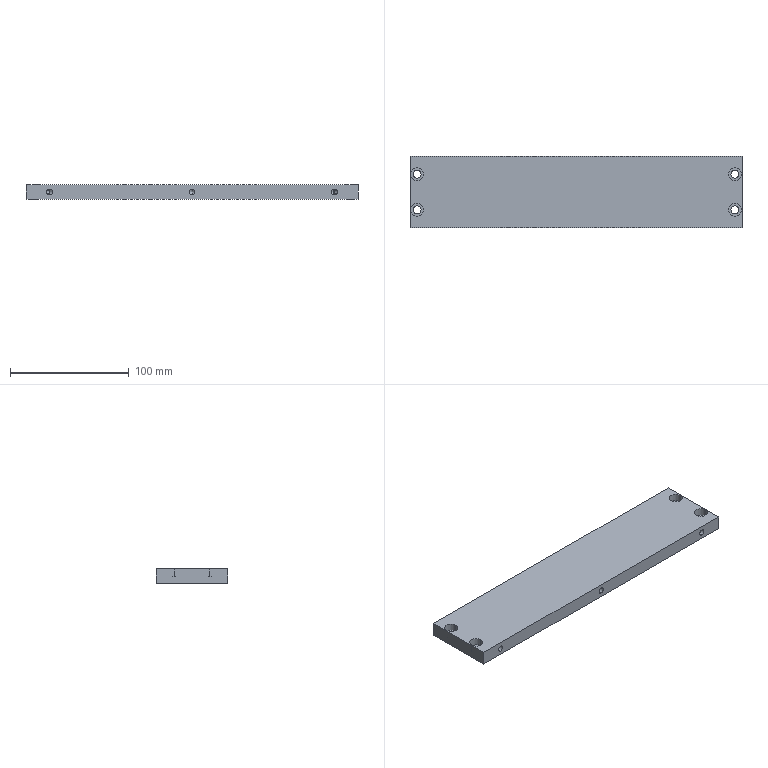Part | SolidWorks | features HoleWzd 3, Extrusion 1 | 1 solid | 50 faces | box 280 x 60 x 12 mm | volume 196575 mm3 | cylinder 28 | cone 12 | plane 10 | commonest cylinder face diameters 5 x12 6.6 x8 11 x8
STEP:
#1=CARTESIAN_POINT('',(268.5,-45.,5.6));
#2=VERTEX_POINT('',#1);
#3=CARTESIAN_POINT('',(279.5,-45.,5.6));
#4=VERTEX_POINT('',#3);
#5=CARTESIAN_POINT('',(274.,-45.,5.6));
#6=DIRECTION('',(0.,0.,1.));
#7=DIRECTION('',(1.,0.,0.));
#8=AXIS2_PLACEMENT_3D('',#5,#6,#7);
#9=CIRCLE('',#8,5.5);
#10=EDGE_CURVE('',#2,#4,#9,.T.);
#11=ORIENTED_EDGE('',*,*,#10,.F.);
#12=CARTESIAN_POINT('',(268.5,-45.,12.));
#13=VERTEX_POINT('',#12);
#14=CARTESIAN_POINT('',(268.5,-45.,12.));
#15=DIRECTION('',(0.,0.,1.));
#16=VECTOR('',#15,1000.);
#17=LINE('',#14,#16);
#18=EDGE_CURVE('',#2,#13,#17,.T.);
#19=ORIENTED_EDGE('',*,*,#18,.T.);
#20=CARTESIAN_POINT('',(279.5,-45.,12.));
#21=VERTEX_POINT('',#20);
#22=CARTESIAN_POINT('',(274.,-45.,12.));
#23=DIRECTION('',(0.,0.,1.));
#24=DIRECTION('',(1.,0.,0.));
#25=AXIS2_PLACEMENT_3D('',#22,#23,#24);
#26=CIRCLE('',#25,5.5);
#27=EDGE_CURVE('',#13,#21,#26,.T.);
#28=ORIENTED_EDGE('',*,*,#27,.T.);
#29=CARTESIAN_POINT('',(279.5,-45.,12.));
#30=DIRECTION('',(0.,0.,1.));
#31=VECTOR('',#30,1000.);
#32=LINE('',#29,#31);
#33=EDGE_CURVE('',#4,#21,#32,.T.);
#34=ORIENTED_EDGE('',*,*,#33,.F.);
#35=EDGE_LOOP('',(#11,#19,#28,#34));
#36=FACE_OUTER_BOUND('',#35,.T.);
#37=CARTESIAN_POINT('',(274.,-45.,12.));
#38=DIRECTION('',(0.,0.,1.));
#39=DIRECTION('',(1.,0.,0.));
#40=AXIS2_PLACEMENT_3D('',#37,#38,#39);
#41=CYLINDRICAL_SURFACE('',#40,5.5);
#42=ADVANCED_FACE('',(#36),#41,.F.);
#43=CARTESIAN_POINT('',(270.7,-45.,0.));
#44=VERTEX_POINT('',#43);
#45=CARTESIAN_POINT('',(277.3,-45.,0.));
#46=VERTEX_POINT('',#45);
#47=CARTESIAN_POINT('',(274.,-45.,0.));
#48=DIRECTION('',(0.,0.,1.));
#49=DIRECTION('',(1.,0.,0.));
#50=AXIS2_PLACEMENT_3D('',#47,#48,#49);
#51=CIRCLE('',#50,3.3);
#52=EDGE_CURVE('',#44,#46,#51,.T.);
#53=ORIENTED_EDGE('',*,*,#52,.F.);
#54=CARTESIAN_POINT('',(270.7,-45.,5.6));
#55=VERTEX_POINT('',#54);
#56=CARTESIAN_POINT('',(270.7,-45.,12.));
#57=DIRECTION('',(0.,0.,1.));
#58=VECTOR('',#57,1000.);
#59=LINE('',#56,#58);
#60=EDGE_CURVE('',#44,#55,#59,.T.);
#61=ORIENTED_EDGE('',*,*,#60,.T.);
#62=CARTESIAN_POINT('',(277.3,-45.,5.6));
#63=VERTEX_POINT('',#62);
#64=CARTESIAN_POINT('',(274.,-45.,5.6));
#65=DIRECTION('',(0.,0.,1.));
#66=DIRECTION('',(1.,0.,0.));
#67=AXIS2_PLACEMENT_3D('',#64,#65,#66);
#68=CIRCLE('',#67,3.3);
#69=EDGE_CURVE('',#55,#63,#68,.T.);
#70=ORIENTED_EDGE('',*,*,#69,.T.);
#71=CARTESIAN_POINT('',(277.3,-45.,12.));
#72=DIRECTION('',(0.,0.,1.));
#73=VECTOR('',#72,1000.);
#74=LINE('',#71,#73);
#75=EDGE_CURVE('',#46,#63,#74,.T.);
#76=ORIENTED_EDGE('',*,*,#75,.F.);
#77=EDGE_LOOP('',(#53,#61,#70,#76));
#78=FACE_OUTER_BOUND('',#77,.T.);
#79=CARTESIAN_POINT('',(274.,-45.,12.));
#80=DIRECTION('',(0.,0.,1.));
#81=DIRECTION('',(1.,0.,0.));
#82=AXIS2_PLACEMENT_3D('',#79,#80,#81);
#83=CYLINDRICAL_SURFACE('',#82,3.3);
#84=ADVANCED_FACE('',(#78),#83,.F.);
#85=CARTESIAN_POINT('',(268.5,-15.,5.6));
#86=VERTEX_POINT('',#85);
#87=CARTESIAN_POINT('',(279.5,-15.,5.6));
#88=VERTEX_POINT('',#87);
#89=CARTESIAN_POINT('',(274.,-15.,5.6));
#90=DIRECTION('',(0.,0.,1.));
#91=DIRECTION('',(1.,0.,0.));
#92=AXIS2_PLACEMENT_3D('',#89,#90,#91);
#93=CIRCLE('',#92,5.5);
#94=EDGE_CURVE('',#86,#88,#93,.T.);
#95=ORIENTED_EDGE('',*,*,#94,.F.);
#96=CARTESIAN_POINT('',(268.5,-15.,12.));
#97=VERTEX_POINT('',#96);
#98=CARTESIAN_POINT('',(268.5,-15.,12.));
#99=DIRECTION('',(0.,0.,1.));
#100=VECTOR('',#99,1000.);
#101=LINE('',#98,#100);
#102=EDGE_CURVE('',#86,#97,#101,.T.);
#103=ORIENTED_EDGE('',*,*,#102,.T.);
#104=CARTESIAN_POINT('',(279.5,-15.,12.));
#105=VERTEX_POINT('',#104);
#106=CARTESIAN_POINT('',(274.,-15.,12.));
#107=DIRECTION('',(0.,0.,1.));
#108=DIRECTION('',(1.,0.,0.));
#109=AXIS2_PLACEMENT_3D('',#106,#107,#108);
#110=CIRCLE('',#109,5.5);
#111=EDGE_CURVE('',#97,#105,#110,.T.);
#112=ORIENTED_EDGE('',*,*,#111,.T.);
#113=CARTESIAN_POINT('',(279.5,-15.,12.));
#114=DIRECTION('',(0.,0.,1.));
#115=VECTOR('',#114,1000.);
#116=LINE('',#113,#115);
#117=EDGE_CURVE('',#88,#105,#116,.T.);
#118=ORIENTED_EDGE('',*,*,#117,.F.);
#119=EDGE_LOOP('',(#95,#103,#112,#118));
#120=FACE_OUTER_BOUND('',#119,.T.);
#121=CARTESIAN_POINT('',(274.,-15.,12.));
#122=DIRECTION('',(0.,0.,1.));
#123=DIRECTION('',(1.,0.,0.));
#124=AXIS2_PLACEMENT_3D('',#121,#122,#123);
#125=CYLINDRICAL_SURFACE('',#124,5.5);
#126=ADVANCED_FACE('',(#120),#125,.F.);
#127=CARTESIAN_POINT('',(270.7,-15.,0.));
#128=VERTEX_POINT('',#127);
#129=CARTESIAN_POINT('',(277.3,-15.,0.));
#130=VERTEX_POINT('',#129);
#131=CARTESIAN_POINT('',(274.,-15.,0.));
#132=DIRECTION('',(0.,0.,1.));
#133=DIRECTION('',(1.,0.,0.));
#134=AXIS2_PLACEMENT_3D('',#131,#132,#133);
#135=CIRCLE('',#134,3.3);
#136=EDGE_CURVE('',#128,#130,#135,.T.);
#137=ORIENTED_EDGE('',*,*,#136,.F.);
#138=CARTESIAN_POINT('',(270.7,-15.,5.6));
#139=VERTEX_POINT('',#138);
#140=CARTESIAN_POINT('',(270.7,-15.,12.));
#141=DIRECTION('',(0.,0.,1.));
#142=VECTOR('',#141,1000.);
#143=LINE('',#140,#142);
#144=EDGE_CURVE('',#128,#139,#143,.T.);
#145=ORIENTED_EDGE('',*,*,#144,.T.);
#146=CARTESIAN_POINT('',(277.3,-15.,5.6));
#147=VERTEX_POINT('',#146);
#148=CARTESIAN_POINT('',(274.,-15.,5.6));
#149=DIRECTION('',(0.,0.,1.));
#150=DIRECTION('',(1.,0.,0.));
#151=AXIS2_PLACEMENT_3D('',#148,#149,#150);
#152=CIRCLE('',#151,3.3);
#153=EDGE_CURVE('',#139,#147,#152,.T.);
#154=ORIENTED_EDGE('',*,*,#153,.T.);
#155=CARTESIAN_POINT('',(277.3,-15.,12.));
#156=DIRECTION('',(0.,0.,1.));
#157=VECTOR('',#156,1000.);
#158=LINE('',#155,#157);
#159=EDGE_CURVE('',#130,#147,#158,.T.);
#160=ORIENTED_EDGE('',*,*,#159,.F.);
#161=EDGE_LOOP('',(#137,#145,#154,#160));
#162=FACE_OUTER_BOUND('',#161,.T.);
#163=CARTESIAN_POINT('',(274.,-15.,12.));
#164=DIRECTION('',(0.,0.,1.));
#165=DIRECTION('',(1.,0.,0.));
#166=AXIS2_PLACEMENT_3D('',#163,#164,#165);
#167=CYLINDRICAL_SURFACE('',#166,3.3);
#168=ADVANCED_FACE('',(#162),#167,.F.);
#169=CARTESIAN_POINT('',(0.5,-45.,5.6));
#170=VERTEX_POINT('',#169);
#171=CARTESIAN_POINT('',(11.5,-45.,5.6));
#172=VERTEX_POINT('',#171);
#173=CARTESIAN_POINT('',(6.,-45.,5.6));
#174=DIRECTION('',(0.,0.,1.));
#175=DIRECTION('',(1.,0.,0.));
#176=AXIS2_PLACEMENT_3D('',#173,#174,#175);
#177=CIRCLE('',#176,5.5);
#178=EDGE_CURVE('',#170,#172,#177,.T.);
#179=ORIENTED_EDGE('',*,*,#178,.F.);
#180=CARTESIAN_POINT('',(0.5,-45.,12.));
#181=VERTEX_POINT('',#180);
#182=CARTESIAN_POINT('',(0.5,-45.,12.));
#183=DIRECTION('',(0.,0.,1.));
#184=VECTOR('',#183,1000.);
#185=LINE('',#182,#184);
#186=EDGE_CURVE('',#170,#181,#185,.T.);
#187=ORIENTED_EDGE('',*,*,#186,.T.);
#188=CARTESIAN_POINT('',(11.5,-45.,12.));
#189=VERTEX_POINT('',#188);
#190=CARTESIAN_POINT('',(6.,-45.,12.));
#191=DIRECTION('',(0.,0.,1.));
#192=DIRECTION('',(1.,0.,0.));
#193=AXIS2_PLACEMENT_3D('',#190,#191,#192);
#194=CIRCLE('',#193,5.5);
#195=EDGE_CURVE('',#181,#189,#194,.T.);
#196=ORIENTED_EDGE('',*,*,#195,.T.);
#197=CARTESIAN_POINT('',(11.5,-45.,12.));
#198=DIRECTION('',(0.,0.,1.));
#199=VECTOR('',#198,1000.);
#200=LINE('',#197,#199);
#201=EDGE_CURVE('',#172,#189,#200,.T.);
#202=ORIENTED_EDGE('',*,*,#201,.F.);
#203=EDGE_LOOP('',(#179,#187,#196,#202));
#204=FACE_OUTER_BOUND('',#203,.T.);
#205=CARTESIAN_POINT('',(6.,-45.,12.));
#206=DIRECTION('',(0.,0.,1.));
#207=DIRECTION('',(1.,0.,0.));
#208=AXIS2_PLACEMENT_3D('',#205,#206,#207);
#209=CYLINDRICAL_SURFACE('',#208,5.5);
#210=ADVANCED_FACE('',(#204),#209,.F.);
#211=CARTESIAN_POINT('',(2.7,-45.,0.));
#212=VERTEX_POINT('',#211);
#213=CARTESIAN_POINT('',(9.3,-45.,0.));
#214=VERTEX_POINT('',#213);
#215=CARTESIAN_POINT('',(6.,-45.,0.));
#216=DIRECTION('',(0.,0.,1.));
#217=DIRECTION('',(1.,0.,0.));
#218=AXIS2_PLACEMENT_3D('',#215,#216,#217);
#219=CIRCLE('',#218,3.3);
#220=EDGE_CURVE('',#212,#214,#219,.T.);
#221=ORIENTED_EDGE('',*,*,#220,.F.);
#222=CARTESIAN_POINT('',(2.7,-45.,5.6));
#223=VERTEX_POINT('',#222);
#224=CARTESIAN_POINT('',(2.7,-45.,12.));
#225=DIRECTION('',(0.,0.,1.));
#226=VECTOR('',#225,1000.);
#227=LINE('',#224,#226);
#228=EDGE_CURVE('',#212,#223,#227,.T.);
#229=ORIENTED_EDGE('',*,*,#228,.T.);
#230=CARTESIAN_POINT('',(9.3,-45.,5.6));
#231=VERTEX_POINT('',#230);
#232=CARTESIAN_POINT('',(6.,-45.,5.6));
#233=DIRECTION('',(0.,0.,1.));
#234=DIRECTION('',(1.,0.,0.));
#235=AXIS2_PLACEMENT_3D('',#232,#233,#234);
#236=CIRCLE('',#235,3.3);
#237=EDGE_CURVE('',#223,#231,#236,.T.);
#238=ORIENTED_EDGE('',*,*,#237,.T.);
#239=CARTESIAN_POINT('',(9.3,-45.,12.));
#240=DIRECTION('',(0.,0.,1.));
#241=VECTOR('',#240,1000.);
#242=LINE('',#239,#241);
#243=EDGE_CURVE('',#214,#231,#242,.T.);
#244=ORIENTED_EDGE('',*,*,#243,.F.);
#245=EDGE_LOOP('',(#221,#229,#238,#244));
#246=FACE_OUTER_BOUND('',#245,.T.);
#247=CARTESIAN_POINT('',(6.,-45.,12.));
#248=DIRECTION('',(0.,0.,1.));
#249=DIRECTION('',(1.,0.,0.));
#250=AXIS2_PLACEMENT_3D('',#247,#248,#249);
#251=CYLINDRICAL_SURFACE('',#250,3.3);
#252=ADVANCED_FACE('',(#246),#251,.F.);
#253=CARTESIAN_POINT('',(0.5,-15.,5.6));
#254=VERTEX_POINT('',#253);
#255=CARTESIAN_POINT('',(11.5,-15.,5.6));
#256=VERTEX_POINT('',#255);
#257=CARTESIAN_POINT('',(6.,-15.,5.6));
#258=DIRECTION('',(0.,0.,1.));
#259=DIRECTION('',(1.,0.,0.));
#260=AXIS2_PLACEMENT_3D('',#257,#258,#259);
#261=CIRCLE('',#260,5.5);
#262=EDGE_CURVE('',#254,#256,#261,.T.);
#263=ORIENTED_EDGE('',*,*,#262,.F.);
#264=CARTESIAN_POINT('',(0.5,-15.,12.));
#265=VERTEX_POINT('',#264);
#266=CARTESIAN_POINT('',(0.5,-15.,12.));
#267=DIRECTION('',(0.,0.,1.));
#268=VECTOR('',#267,1000.);
#269=LINE('',#266,#268);
#270=EDGE_CURVE('',#254,#265,#269,.T.);
#271=ORIENTED_EDGE('',*,*,#270,.T.);
#272=CARTESIAN_POINT('',(11.5,-15.,12.));
#273=VERTEX_POINT('',#272);
#274=CARTESIAN_POINT('',(6.,-15.,12.));
#275=DIRECTION('',(0.,0.,1.));
#276=DIRECTION('',(1.,0.,0.));
#277=AXIS2_PLACEMENT_3D('',#274,#275,#276);
#278=CIRCLE('',#277,5.5);
#279=EDGE_CURVE('',#265,#273,#278,.T.);
#280=ORIENTED_EDGE('',*,*,#279,.T.);
#281=CARTESIAN_POINT('',(11.5,-15.,12.));
#282=DIRECTION('',(0.,0.,1.));
#283=VECTOR('',#282,1000.);
#284=LINE('',#281,#283);
#285=EDGE_CURVE('',#256,#273,#284,.T.);
#286=ORIENTED_EDGE('',*,*,#285,.F.);
#287=EDGE_LOOP('',(#263,#271,#280,#286));
#288=FACE_OUTER_BOUND('',#287,.T.);
#289=CARTESIAN_POINT('',(6.,-15.,12.));
#290=DIRECTION('',(0.,0.,1.));
#291=DIRECTION('',(1.,0.,0.));
#292=AXIS2_PLACEMENT_3D('',#289,#290,#291);
#293=CYLINDRICAL_SURFACE('',#292,5.5);
#294=ADVANCED_FACE('',(#288),#293,.F.);
#295=CARTESIAN_POINT('',(2.7,-15.,0.));
#296=VERTEX_POINT('',#295);
#297=CARTESIAN_POINT('',(9.3,-15.,0.));
#298=VERTEX_POINT('',#297);
#299=CARTESIAN_POINT('',(6.,-15.,0.));
#300=DIRECTION('',(0.,0.,1.));
#301=DIRECTION('',(1.,0.,0.));
#302=AXIS2_PLACEMENT_3D('',#299,#300,#301);
#303=CIRCLE('',#302,3.3);
#304=EDGE_CURVE('',#296,#298,#303,.T.);
#305=ORIENTED_EDGE('',*,*,#304,.F.);
#306=CARTESIAN_POINT('',(2.7,-15.,5.6));
#307=VERTEX_POINT('',#306);
#308=CARTESIAN_POINT('',(2.7,-15.,12.));
#309=DIRECTION('',(0.,0.,1.));
#310=VECTOR('',#309,1000.);
#311=LINE('',#308,#310);
#312=EDGE_CURVE('',#296,#307,#311,.T.);
#313=ORIENTED_EDGE('',*,*,#312,.T.);
#314=CARTESIAN_POINT('',(9.3,-15.,5.6));
#315=VERTEX_POINT('',#314);
#316=CARTESIAN_POINT('',(6.,-15.,5.6));
#317=DIRECTION('',(0.,0.,1.));
#318=DIRECTION('',(1.,0.,0.));
#319=AXIS2_PLACEMENT_3D('',#316,#317,#318);
#320=CIRCLE('',#319,3.3);
#321=EDGE_CURVE('',#307,#315,#320,.T.);
#322=ORIENTED_EDGE('',*,*,#321,.T.);
#323=CARTESIAN_POINT('',(9.3,-15.,12.));
#324=DIRECTION('',(0.,0.,1.));
#325=VECTOR('',#324,1000.);
#326=LINE('',#323,#325);
#327=EDGE_CURVE('',#298,#315,#326,.T.);
#328=ORIENTED_EDGE('',*,*,#327,.F.);
#329=EDGE_LOOP('',(#305,#313,#322,#328));
#330=FACE_OUTER_BOUND('',#329,.T.);
#331=CARTESIAN_POINT('',(6.,-15.,12.));
#332=DIRECTION('',(0.,0.,1.));
#333=DIRECTION('',(1.,0.,0.));
#334=AXIS2_PLACEMENT_3D('',#331,#332,#333);
#335=CYLINDRICAL_SURFACE('',#334,3.3);
#336=ADVANCED_FACE('',(#330),#335,.F.);
#337=CARTESIAN_POINT('',(260.,-45.,8.5));
#338=VERTEX_POINT('',#337);
#339=CARTESIAN_POINT('',(260.,-45.,3.5));
#340=VERTEX_POINT('',#339);
#341=CARTESIAN_POINT('',(260.,-45.,6.));
#342=DIRECTION('',(0.,-1.,0.));
#343=DIRECTION('',(0.,0.,-1.));
#344=AXIS2_PLACEMENT_3D('',#341,#342,#343);
#345=CIRCLE('',#344,2.5);
#346=EDGE_CURVE('',#338,#340,#345,.T.);
#347=ORIENTED_EDGE('',*,*,#346,.F.);
#348=CARTESIAN_POINT('',(260.,-60.,8.5));
#349=VERTEX_POINT('',#348);
#350=CARTESIAN_POINT('',(260.,-60.,8.5));
#351=DIRECTION('',(0.,-1.,0.));
#352=VECTOR('',#351,1000.);
#353=LINE('',#350,#352);
#354=EDGE_CURVE('',#338,#349,#353,.T.);
#355=ORIENTED_EDGE('',*,*,#354,.T.);
#356=CARTESIAN_POINT('',(260.,-60.,3.5));
#357=VERTEX_POINT('',#356);
#358=CARTESIAN_POINT('',(260.,-60.,6.));
#359=DIRECTION('',(0.,-1.,0.));
#360=DIRECTION('',(0.,0.,-1.));
#361=AXIS2_PLACEMENT_3D('',#358,#359,#360);
#362=CIRCLE('',#361,2.5);
#363=EDGE_CURVE('',#349,#357,#362,.T.);
#364=ORIENTED_EDGE('',*,*,#363,.T.);
#365=CARTESIAN_POINT('',(260.,-60.,3.5));
#366=DIRECTION('',(0.,-1.,0.));
#367=VECTOR('',#366,1000.);
#368=LINE('',#365,#367);
#369=EDGE_CURVE('',#340,#357,#368,.T.);
#370=ORIENTED_EDGE('',*,*,#369,.F.);
#371=EDGE_LOOP('',(#347,#355,#364,#370));
#372=FACE_OUTER_BOUND('',#371,.T.);
#373=CARTESIAN_POINT('',(260.,-60.,6.));
#374=DIRECTION('',(0.,-1.,0.));
#375=DIRECTION('',(0.,0.,-1.));
#376=AXIS2_PLACEMENT_3D('',#373,#374,#375);
#377=CYLINDRICAL_SURFACE('',#376,2.5);
#378=ADVANCED_FACE('',(#372),#377,.F.);
#379=CARTESIAN_POINT('',(260.,-43.498,6.));
#380=VERTEX_POINT('',#379);
#381=CARTESIAN_POINT('',(260.,-45.,3.5));
#382=DIRECTION('',(0.,-0.515,-0.8572));
#383=VECTOR('',#382,1000.);
#384=LINE('',#381,#383);
#385=EDGE_CURVE('',#380,#340,#384,.T.);
#386=ORIENTED_EDGE('',*,*,#385,.F.);
#387=CARTESIAN_POINT('',(260.,-45.,8.5));
#388=DIRECTION('',(0.,-0.515,0.8572));
#389=VECTOR('',#388,1000.);
#390=LINE('',#387,#389);
#391=EDGE_CURVE('',#380,#338,#390,.T.);
#392=ORIENTED_EDGE('',*,*,#391,.T.);
#393=ORIENTED_EDGE('',*,*,#346,.T.);
#394=EDGE_LOOP('',(#386,#392,#393));
#395=FACE_OUTER_BOUND('',#394,.T.);
#396=CARTESIAN_POINT('',(260.,-45.,6.));
#397=DIRECTION('',(0.,-1.,0.));
#398=DIRECTION('',(0.,0.,-1.));
#399=AXIS2_PLACEMENT_3D('',#396,#397,#398);
#400=CONICAL_SURFACE('',#399,2.5,1.03);
#401=ADVANCED_FACE('',(#395),#400,.F.);
#402=CARTESIAN_POINT('',(140.,-45.,8.5));
#403=VERTEX_POINT('',#402);
#404=CARTESIAN_POINT('',(140.,-45.,3.5));
#405=VERTEX_POINT('',#404);
#406=CARTESIAN_POINT('',(140.,-45.,6.));
#407=DIRECTION('',(0.,-1.,0.));
#408=DIRECTION('',(0.,0.,-1.));
#409=AXIS2_PLACEMENT_3D('',#406,#407,#408);
#410=CIRCLE('',#409,2.5);
#411=EDGE_CURVE('',#403,#405,#410,.T.);
#412=ORIENTED_EDGE('',*,*,#411,.F.);
#413=CARTESIAN_POINT('',(140.,-60.,8.5));
#414=VERTEX_POINT('',#413);
#415=CARTESIAN_POINT('',(140.,-60.,8.5));
#416=DIRECTION('',(0.,-1.,0.));
#417=VECTOR('',#416,1000.);
#418=LINE('',#415,#417);
#419=EDGE_CURVE('',#403,#414,#418,.T.);
#420=ORIENTED_EDGE('',*,*,#419,.T.);
#421=CARTESIAN_POINT('',(140.,-60.,3.5));
#422=VERTEX_POINT('',#421);
#423=CARTESIAN_POINT('',(140.,-60.,6.));
#424=DIRECTION('',(0.,-1.,0.));
#425=DIRECTION('',(0.,0.,-1.));
#426=AXIS2_PLACEMENT_3D('',#423,#424,#425);
#427=CIRCLE('',#426,2.5);
#428=EDGE_CURVE('',#414,#422,#427,.T.);
#429=ORIENTED_EDGE('',*,*,#428,.T.);
#430=CARTESIAN_POINT('',(140.,-60.,3.5));
#431=DIRECTION('',(0.,-1.,0.));
#432=VECTOR('',#431,1000.);
#433=LINE('',#430,#432);
#434=EDGE_CURVE('',#405,#422,#433,.T.);
#435=ORIENTED_EDGE('',*,*,#434,.F.);
#436=EDGE_LOOP('',(#412,#420,#429,#435));
#437=FACE_OUTER_BOUND('',#436,.T.);
#438=CARTESIAN_POINT('',(140.,-60.,6.));
#439=DIRECTION('',(0.,-1.,0.));
#440=DIRECTION('',(0.,0.,-1.));
#441=AXIS2_PLACEMENT_3D('',#438,#439,#440);
#442=CYLINDRICAL_SURFACE('',#441,2.5);
#443=ADVANCED_FACE('',(#437),#442,.F.);
#444=CARTESIAN_POINT('',(140.,-43.498,6.));
#445=VERTEX_POINT('',#444);
#446=CARTESIAN_POINT('',(140.,-45.,3.5));
#447=DIRECTION('',(0.,-0.515,-0.8572));
#448=VECTOR('',#447,1000.);
#449=LINE('',#446,#448);
#450=EDGE_CURVE('',#445,#405,#449,.T.);
#451=ORIENTED_EDGE('',*,*,#450,.F.);
#452=CARTESIAN_POINT('',(140.,-45.,8.5));
#453=DIRECTION('',(0.,-0.515,0.8572));
#454=VECTOR('',#453,1000.);
#455=LINE('',#452,#454);
#456=EDGE_CURVE('',#445,#403,#455,.T.);
#457=ORIENTED_EDGE('',*,*,#456,.T.);
#458=ORIENTED_EDGE('',*,*,#411,.T.);
#459=EDGE_LOOP('',(#451,#457,#458));
#460=FACE_OUTER_BOUND('',#459,.T.);
#461=CARTESIAN_POINT('',(140.,-45.,6.));
#462=DIRECTION('',(0.,-1.,0.));
#463=DIRECTION('',(0.,0.,-1.));
#464=AXIS2_PLACEMENT_3D('',#461,#462,#463);
#465=CONICAL_SURFACE('',#464,2.5,1.03);
#466=ADVANCED_FACE('',(#460),#465,.F.);
#467=CARTESIAN_POINT('',(20.,-45.,8.5));
#468=VERTEX_POINT('',#467);
#469=CARTESIAN_POINT('',(20.,-45.,3.5));
#470=VERTEX_POINT('',#469);
#471=CARTESIAN_POINT('',(20.,-45.,6.));
#472=DIRECTION('',(0.,-1.,0.));
#473=DIRECTION('',(0.,0.,-1.));
#474=AXIS2_PLACEMENT_3D('',#471,#472,#473);
#475=CIRCLE('',#474,2.5);
#476=EDGE_CURVE('',#468,#470,#475,.T.);
#477=ORIENTED_EDGE('',*,*,#476,.F.);
#478=CARTESIAN_POINT('',(20.,-60.,8.5));
#479=VERTEX_POINT('',#478);
#480=CARTESIAN_POINT('',(20.,-60.,8.5));
#481=DIRECTION('',(0.,-1.,0.));
#482=VECTOR('',#481,1000.);
#483=LINE('',#480,#482);
#484=EDGE_CURVE('',#468,#479,#483,.T.);
#485=ORIENTED_EDGE('',*,*,#484,.T.);
#486=CARTESIAN_POINT('',(20.,-60.,3.5));
#487=VERTEX_POINT('',#486);
#488=CARTESIAN_POINT('',(20.,-60.,6.));
#489=DIRECTION('',(0.,-1.,0.));
#490=DIRECTION('',(0.,0.,-1.));
#491=AXIS2_PLACEMENT_3D('',#488,#489,#490);
#492=CIRCLE('',#491,2.5);
#493=EDGE_CURVE('',#479,#487,#492,.T.);
#494=ORIENTED_EDGE('',*,*,#493,.T.);
#495=CARTESIAN_POINT('',(20.,-60.,3.5));
#496=DIRECTION('',(0.,-1.,0.));
#497=VECTOR('',#496,1000.);
#498=LINE('',#495,#497);
#499=EDGE_CURVE('',#470,#487,#498,.T.);
#500=ORIENTED_EDGE('',*,*,#499,.F.);
#501=EDGE_LOOP('',(#477,#485,#494,#500));
#502=FACE_OUTER_BOUND('',#501,.T.);
#503=CARTESIAN_POINT('',(20.,-60.,6.));
#504=DIRECTION('',(0.,-1.,0.));
#505=DIRECTION('',(0.,0.,-1.));
#506=AXIS2_PLACEMENT_3D('',#503,#504,#505);
#507=CYLINDRICAL_SURFACE('',#506,2.5);
#508=ADVANCED_FACE('',(#502),#507,.F.);
#509=CARTESIAN_POINT('',(20.,-43.498,6.));
#510=VERTEX_POINT('',#509);
#511=CARTESIAN_POINT('',(20.,-45.,3.5));
#512=DIRECTION('',(0.,-0.515,-0.8572));
#513=VECTOR('',#512,1000.);
#514=LINE('',#511,#513);
#515=EDGE_CURVE('',#510,#470,#514,.T.);
#516=ORIENTED_EDGE('',*,*,#515,.F.);
#517=CARTESIAN_POINT('',(20.,-45.,8.5));
#518=DIRECTION('',(0.,-0.515,0.8572));
#519=VECTOR('',#518,1000.);
#520=LINE('',#517,#519);
#521=EDGE_CURVE('',#510,#468,#520,.T.);
#522=ORIENTED_EDGE('',*,*,#521,.T.);
#523=ORIENTED_EDGE('',*,*,#476,.T.);
#524=EDGE_LOOP('',(#516,#522,#523));
#525=FACE_OUTER_BOUND('',#524,.T.);
#526=CARTESIAN_POINT('',(20.,-45.,6.));
#527=DIRECTION('',(0.,-1.,0.));
#528=DIRECTION('',(0.,0.,-1.));
#529=AXIS2_PLACEMENT_3D('',#526,#527,#528);
#530=CONICAL_SURFACE('',#529,2.5,1.03);
#531=ADVANCED_FACE('',(#525),#530,.F.);
#532=CARTESIAN_POINT('',(260.,-15.,3.5));
#533=VERTEX_POINT('',#532);
#534=CARTESIAN_POINT('',(260.,-15.,8.5));
#535=VERTEX_POINT('',#534);
#536=CARTESIAN_POINT('',(260.,-15.,6.));
#537=DIRECTION('',(0.,1.,0.));
#538=DIRECTION('',(0.,0.,1.));
#539=AXIS2_PLACEMENT_3D('',#536,#537,#538);
#540=CIRCLE('',#539,2.5);
#541=EDGE_CURVE('',#533,#535,#540,.T.);
#542=ORIENTED_EDGE('',*,*,#541,.F.);
#543=CARTESIAN_POINT('',(260.,0.,3.5));
#544=VERTEX_POINT('',#543);
#545=CARTESIAN_POINT('',(260.,0.,3.5));
#546=DIRECTION('',(0.,1.,0.));
#547=VECTOR('',#546,1000.);
#548=LINE('',#545,#547);
#549=EDGE_CURVE('',#533,#544,#548,.T.);
#550=ORIENTED_EDGE('',*,*,#549,.T.);
#551=CARTESIAN_POINT('',(260.,0.,8.5));
#552=VERTEX_POINT('',#551);
#553=CARTESIAN_POINT('',(260.,0.,6.));
#554=DIRECTION('',(0.,1.,0.));
#555=DIRECTION('',(0.,0.,1.));
#556=AXIS2_PLACEMENT_3D('',#553,#554,#555);
#557=CIRCLE('',#556,2.5);
#558=EDGE_CURVE('',#544,#552,#557,.T.);
#559=ORIENTED_EDGE('',*,*,#558,.T.);
#560=CARTESIAN_POINT('',(260.,0.,8.5));
#561=DIRECTION('',(0.,1.,0.));
#562=VECTOR('',#561,1000.);
#563=LINE('',#560,#562);
#564=EDGE_CURVE('',#535,#552,#563,.T.);
#565=ORIENTED_EDGE('',*,*,#564,.F.);
#566=EDGE_LOOP('',(#542,#550,#559,#565));
#567=FACE_OUTER_BOUND('',#566,.T.);
#568=CARTESIAN_POINT('',(260.,0.,6.));
#569=DIRECTION('',(0.,1.,0.));
#570=DIRECTION('',(0.,0.,1.));
#571=AXIS2_PLACEMENT_3D('',#568,#569,#570);
#572=CYLINDRICAL_SURFACE('',#571,2.5);
#573=ADVANCED_FACE('',(#567),#572,.F.);
#574=CARTESIAN_POINT('',(260.,-16.502,6.));
#575=VERTEX_POINT('',#574);
#576=CARTESIAN_POINT('',(260.,-15.,8.5));
#577=DIRECTION('',(0.,0.515,0.8572));
#578=VECTOR('',#577,1000.);
#579=LINE('',#576,#578);
#580=EDGE_CURVE('',#575,#535,#579,.T.);
#581=ORIENTED_EDGE('',*,*,#580,.F.);
#582=CARTESIAN_POINT('',(260.,-15.,3.5));
#583=DIRECTION('',(0.,0.515,-0.8572));
#584=VECTOR('',#583,1000.);
#585=LINE('',#582,#584);
#586=EDGE_CURVE('',#575,#533,#585,.T.);
#587=ORIENTED_EDGE('',*,*,#586,.T.);
#588=ORIENTED_EDGE('',*,*,#541,.T.);
#589=EDGE_LOOP('',(#581,#587,#588));
#590=FACE_OUTER_BOUND('',#589,.T.);
#591=CARTESIAN_POINT('',(260.,-15.,6.));
#592=DIRECTION('',(0.,1.,0.));
#593=DIRECTION('',(0.,0.,1.));
#594=AXIS2_PLACEMENT_3D('',#591,#592,#593);
#595=CONICAL_SURFACE('',#594,2.5,1.03);
#596=ADVANCED_FACE('',(#590),#595,.F.);
#597=CARTESIAN_POINT('',(140.,-15.,3.5));
#598=VERTEX_POINT('',#597);
#599=CARTESIAN_POINT('',(140.,-15.,8.5));
#600=VERTEX_POINT('',#599);
#601=CARTESIAN_POINT('',(140.,-15.,6.));
#602=DIRECTION('',(0.,1.,0.));
#603=DIRECTION('',(0.,0.,1.));
#604=AXIS2_PLACEMENT_3D('',#601,#602,#603);
#605=CIRCLE('',#604,2.5);
#606=EDGE_CURVE('',#598,#600,#605,.T.);
#607=ORIENTED_EDGE('',*,*,#606,.F.);
#608=CARTESIAN_POINT('',(140.,0.,3.5));
#609=VERTEX_POINT('',#608);
#610=CARTESIAN_POINT('',(140.,0.,3.5));
#611=DIRECTION('',(0.,1.,0.));
#612=VECTOR('',#611,1000.);
#613=LINE('',#610,#612);
#614=EDGE_CURVE('',#598,#609,#613,.T.);
#615=ORIENTED_EDGE('',*,*,#614,.T.);
#616=CARTESIAN_POINT('',(140.,0.,8.5));
#617=VERTEX_POINT('',#616);
#618=CARTESIAN_POINT('',(140.,0.,6.));
#619=DIRECTION('',(0.,1.,0.));
#620=DIRECTION('',(0.,0.,1.));
#621=AXIS2_PLACEMENT_3D('',#618,#619,#620);
#622=CIRCLE('',#621,2.5);
#623=EDGE_CURVE('',#609,#617,#622,.T.);
#624=ORIENTED_EDGE('',*,*,#623,.T.);
#625=CARTESIAN_POINT('',(140.,0.,8.5));
#626=DIRECTION('',(0.,1.,0.));
#627=VECTOR('',#626,1000.);
#628=LINE('',#625,#627);
#629=EDGE_CURVE('',#600,#617,#628,.T.);
#630=ORIENTED_EDGE('',*,*,#629,.F.);
#631=EDGE_LOOP('',(#607,#615,#624,#630));
#632=FACE_OUTER_BOUND('',#631,.T.);
#633=CARTESIAN_POINT('',(140.,0.,6.));
#634=DIRECTION('',(0.,1.,0.));
#635=DIRECTION('',(0.,0.,1.));
#636=AXIS2_PLACEMENT_3D('',#633,#634,#635);
#637=CYLINDRICAL_SURFACE('',#636,2.5);
#638=ADVANCED_FACE('',(#632),#637,.F.);
#639=CARTESIAN_POINT('',(140.,-16.502,6.));
#640=VERTEX_POINT('',#639);
#641=CARTESIAN_POINT('',(140.,-15.,8.5));
#642=DIRECTION('',(0.,0.515,0.8572));
#643=VECTOR('',#642,1000.);
#644=LINE('',#641,#643);
#645=EDGE_CURVE('',#640,#600,#644,.T.);
#646=ORIENTED_EDGE('',*,*,#645,.F.);
#647=CARTESIAN_POINT('',(140.,-15.,3.5));
#648=DIRECTION('',(0.,0.515,-0.8572));
#649=VECTOR('',#648,1000.);
#650=LINE('',#647,#649);
#651=EDGE_CURVE('',#640,#598,#650,.T.);
#652=ORIENTED_EDGE('',*,*,#651,.T.);
#653=ORIENTED_EDGE('',*,*,#606,.T.);
#654=EDGE_LOOP('',(#646,#652,#653));
#655=FACE_OUTER_BOUND('',#654,.T.);
#656=CARTESIAN_POINT('',(140.,-15.,6.));
#657=DIRECTION('',(0.,1.,0.));
#658=DIRECTION('',(0.,0.,1.));
#659=AXIS2_PLACEMENT_3D('',#656,#657,#658);
#660=CONICAL_SURFACE('',#659,2.5,1.03);
#661=ADVANCED_FACE('',(#655),#660,.F.);
#662=CARTESIAN_POINT('',(20.,-15.,3.5));
#663=VERTEX_POINT('',#662);
#664=CARTESIAN_POINT('',(20.,-15.,8.5));
#665=VERTEX_POINT('',#664);
#666=CARTESIAN_POINT('',(20.,-15.,6.));
#667=DIRECTION('',(0.,1.,0.));
#668=DIRECTION('',(0.,0.,1.));
#669=AXIS2_PLACEMENT_3D('',#666,#667,#668);
#670=CIRCLE('',#669,2.5);
#671=EDGE_CURVE('',#663,#665,#670,.T.);
#672=ORIENTED_EDGE('',*,*,#671,.F.);
#673=CARTESIAN_POINT('',(20.,0.,3.5));
#674=VERTEX_POINT('',#673);
#675=CARTESIAN_POINT('',(20.,0.,3.5));
#676=DIRECTION('',(0.,1.,0.));
#677=VECTOR('',#676,1000.);
#678=LINE('',#675,#677);
#679=EDGE_CURVE('',#663,#674,#678,.T.);
#680=ORIENTED_EDGE('',*,*,#679,.T.);
#681=CARTESIAN_POINT('',(20.,0.,8.5));
#682=VERTEX_POINT('',#681);
#683=CARTESIAN_POINT('',(20.,0.,6.));
#684=DIRECTION('',(0.,1.,0.));
#685=DIRECTION('',(0.,0.,1.));
#686=AXIS2_PLACEMENT_3D('',#683,#684,#685);
#687=CIRCLE('',#686,2.5);
#688=EDGE_CURVE('',#674,#682,#687,.T.);
#689=ORIENTED_EDGE('',*,*,#688,.T.);
#690=CARTESIAN_POINT('',(20.,0.,8.5));
#691=DIRECTION('',(0.,1.,0.));
#692=VECTOR('',#691,1000.);
#693=LINE('',#690,#692);
#694=EDGE_CURVE('',#665,#682,#693,.T.);
#695=ORIENTED_EDGE('',*,*,#694,.F.);
#696=EDGE_LOOP('',(#672,#680,#689,#695));
#697=FACE_OUTER_BOUND('',#696,.T.);
#698=CARTESIAN_POINT('',(20.,0.,6.));
#699=DIRECTION('',(0.,1.,0.));
#700=DIRECTION('',(0.,0.,1.));
#701=AXIS2_PLACEMENT_3D('',#698,#699,#700);
#702=CYLINDRICAL_SURFACE('',#701,2.5);
#703=ADVANCED_FACE('',(#697),#702,.F.);
#704=CARTESIAN_POINT('',(20.,-16.502,6.));
#705=VERTEX_POINT('',#704);
#706=CARTESIAN_POINT('',(20.,-15.,8.5));
#707=DIRECTION('',(0.,0.515,0.8572));
#708=VECTOR('',#707,1000.);
#709=LINE('',#706,#708);
#710=EDGE_CURVE('',#705,#665,#709,.T.);
#711=ORIENTED_EDGE('',*,*,#710,.F.);
#712=CARTESIAN_POINT('',(20.,-15.,3.5));
#713=DIRECTION('',(0.,0.515,-0.8572));
#714=VECTOR('',#713,1000.);
#715=LINE('',#712,#714);
#716=EDGE_CURVE('',#705,#663,#715,.T.);
#717=ORIENTED_EDGE('',*,*,#716,.T.);
#718=ORIENTED_EDGE('',*,*,#671,.T.);
#719=EDGE_LOOP('',(#711,#717,#718));
#720=FACE_OUTER_BOUND('',#719,.T.);
#721=CARTESIAN_POINT('',(20.,-15.,6.));
#722=DIRECTION('',(0.,1.,0.));
#723=DIRECTION('',(0.,0.,1.));
#724=AXIS2_PLACEMENT_3D('',#721,#722,#723);
#725=CONICAL_SURFACE('',#724,2.5,1.03);
#726=ADVANCED_FACE('',(#720),#725,.F.);
#727=CARTESIAN_POINT('',(0.,0.,0.));
#728=VERTEX_POINT('',#727);
#729=CARTESIAN_POINT('',(0.,-60.,0.));
#730=VERTEX_POINT('',#729);
#731=CARTESIAN_POINT('',(0.,0.,0.));
#732=DIRECTION('',(0.,-1.,0.));
#733=VECTOR('',#732,1000.);
#734=LINE('',#731,#733);
#735=EDGE_CURVE('',#728,#730,#734,.T.);
#736=ORIENTED_EDGE('',*,*,#735,.T.);
#737=CARTESIAN_POINT('',(0.,-60.,12.));
#738=VERTEX_POINT('',#737);
#739=CARTESIAN_POINT('',(0.,-60.,12.));
#740=DIRECTION('',(0.,0.,-1.));
#741=VECTOR('',#740,1000.);
#742=LINE('',#739,#741);
#743=EDGE_CURVE('',#738,#730,#742,.T.);
#744=ORIENTED_EDGE('',*,*,#743,.F.);
#745=CARTESIAN_POINT('',(0.,0.,12.));
#746=VERTEX_POINT('',#745);
#747=CARTESIAN_POINT('',(0.,0.,12.));
#748=DIRECTION('',(0.,-1.,0.));
#749=VECTOR('',#748,1000.);
#750=LINE('',#747,#749);
#751=EDGE_CURVE('',#746,#738,#750,.T.);
#752=ORIENTED_EDGE('',*,*,#751,.F.);
#753=CARTESIAN_POINT('',(0.,0.,12.));
#754=DIRECTION('',(0.,0.,-1.));
#755=VECTOR('',#754,1000.);
#756=LINE('',#753,#755);
#757=EDGE_CURVE('',#746,#728,#756,.T.);
#758=ORIENTED_EDGE('',*,*,#757,.T.);
#759=EDGE_LOOP('',(#736,#744,#752,#758));
#760=FACE_OUTER_BOUND('',#759,.T.);
#761=CARTESIAN_POINT('',(0.,0.,12.));
#762=DIRECTION('',(1.,0.,0.));
#763=DIRECTION('',(0.,1.,0.));
#764=AXIS2_PLACEMENT_3D('',#761,#762,#763);
#765=PLANE('',#764);
#766=ADVANCED_FACE('',(#760),#765,.F.);
#767=CARTESIAN_POINT('',(260.,-60.,6.));
#768=DIRECTION('',(0.,-1.,0.));
#769=DIRECTION('',(0.,0.,-1.));
#770=AXIS2_PLACEMENT_3D('',#767,#768,#769);
#771=CIRCLE('',#770,2.5);
#772=EDGE_CURVE('',#357,#349,#771,.T.);
#773=ORIENTED_EDGE('',*,*,#772,.F.);
#774=ORIENTED_EDGE('',*,*,#363,.F.);
#775=EDGE_LOOP('',(#773,#774));
#776=FACE_BOUND('',#775,.T.);
#777=CARTESIAN_POINT('',(140.,-60.,6.));
#778=DIRECTION('',(0.,-1.,0.));
#779=DIRECTION('',(0.,0.,-1.));
#780=AXIS2_PLACEMENT_3D('',#777,#778,#779);
#781=CIRCLE('',#780,2.5);
#782=EDGE_CURVE('',#422,#414,#781,.T.);
#783=ORIENTED_EDGE('',*,*,#782,.F.);
#784=ORIENTED_EDGE('',*,*,#428,.F.);
#785=EDGE_LOOP('',(#783,#784));
#786=FACE_BOUND('',#785,.T.);
#787=CARTESIAN_POINT('',(20.,-60.,6.));
#788=DIRECTION('',(0.,-1.,0.));
#789=DIRECTION('',(0.,0.,-1.));
#790=AXIS2_PLACEMENT_3D('',#787,#788,#789);
#791=CIRCLE('',#790,2.5);
#792=EDGE_CURVE('',#487,#479,#791,.T.);
#793=ORIENTED_EDGE('',*,*,#792,.F.);
#794=ORIENTED_EDGE('',*,*,#493,.F.);
#795=EDGE_LOOP('',(#793,#794));
#796=FACE_BOUND('',#795,.T.);
#797=CARTESIAN_POINT('',(280.,-60.,0.));
#798=VERTEX_POINT('',#797);
#799=CARTESIAN_POINT('',(0.,-60.,0.));
#800=DIRECTION('',(1.,0.,0.));
#801=VECTOR('',#800,1000.);
#802=LINE('',#799,#801);
#803=EDGE_CURVE('',#730,#798,#802,.T.);
#804=ORIENTED_EDGE('',*,*,#803,.T.);
#805=CARTESIAN_POINT('',(280.,-60.,12.));
#806=VERTEX_POINT('',#805);
#807=CARTESIAN_POINT('',(280.,-60.,12.));
#808=DIRECTION('',(0.,0.,-1.));
#809=VECTOR('',#808,1000.);
#810=LINE('',#807,#809);
#811=EDGE_CURVE('',#806,#798,#810,.T.);
#812=ORIENTED_EDGE('',*,*,#811,.F.);
#813=CARTESIAN_POINT('',(0.,-60.,12.));
#814=DIRECTION('',(1.,0.,0.));
#815=VECTOR('',#814,1000.);
#816=LINE('',#813,#815);
#817=EDGE_CURVE('',#738,#806,#816,.T.);
#818=ORIENTED_EDGE('',*,*,#817,.F.);
#819=ORIENTED_EDGE('',*,*,#743,.T.);
#820=EDGE_LOOP('',(#804,#812,#818,#819));
#821=FACE_OUTER_BOUND('',#820,.T.);
#822=CARTESIAN_POINT('',(0.,-60.,12.));
#823=DIRECTION('',(0.,1.,0.));
#824=DIRECTION('',(0.,0.,1.));
#825=AXIS2_PLACEMENT_3D('',#822,#823,#824);
#826=PLANE('',#825);
#827=ADVANCED_FACE('',(#776,#786,#796,#821),#826,.F.);
#828=CARTESIAN_POINT('',(280.,0.,0.));
#829=VERTEX_POINT('',#828);
#830=CARTESIAN_POINT('',(280.,0.,0.));
#831=DIRECTION('',(0.,1.,0.));
#832=VECTOR('',#831,1000.);
#833=LINE('',#830,#832);
#834=EDGE_CURVE('',#798,#829,#833,.T.);
#835=ORIENTED_EDGE('',*,*,#834,.T.);
#836=CARTESIAN_POINT('',(280.,0.,12.));
#837=VERTEX_POINT('',#836);
#838=CARTESIAN_POINT('',(280.,0.,12.));
#839=DIRECTION('',(0.,0.,-1.));
#840=VECTOR('',#839,1000.);
#841=LINE('',#838,#840);
#842=EDGE_CURVE('',#837,#829,#841,.T.);
#843=ORIENTED_EDGE('',*,*,#842,.F.);
#844=CARTESIAN_POINT('',(280.,0.,12.));
#845=DIRECTION('',(0.,1.,0.));
#846=VECTOR('',#845,1000.);
#847=LINE('',#844,#846);
#848=EDGE_CURVE('',#806,#837,#847,.T.);
#849=ORIENTED_EDGE('',*,*,#848,.F.);
#850=ORIENTED_EDGE('',*,*,#811,.T.);
#851=EDGE_LOOP('',(#835,#843,#849,#850));
#852=FACE_OUTER_BOUND('',#851,.T.);
#853=CARTESIAN_POINT('',(280.,0.,12.));
#854=DIRECTION('',(-1.,0.,0.));
#855=DIRECTION('',(0.,0.,1.));
#856=AXIS2_PLACEMENT_3D('',#853,#854,#855);
#857=PLANE('',#856);
#858=ADVANCED_FACE('',(#852),#857,.F.);
#859=CARTESIAN_POINT('',(260.,0.,6.));
#860=DIRECTION('',(0.,1.,0.));
#861=DIRECTION('',(0.,0.,1.));
#862=AXIS2_PLACEMENT_3D('',#859,#860,#861);
#863=CIRCLE('',#862,2.5);
#864=EDGE_CURVE('',#552,#544,#863,.T.);
#865=ORIENTED_EDGE('',*,*,#864,.F.);
#866=ORIENTED_EDGE('',*,*,#558,.F.);
#867=EDGE_LOOP('',(#865,#866));
#868=FACE_BOUND('',#867,.T.);
#869=CARTESIAN_POINT('',(140.,0.,6.));
#870=DIRECTION('',(0.,1.,0.));
#871=DIRECTION('',(0.,0.,1.));
#872=AXIS2_PLACEMENT_3D('',#869,#870,#871);
#873=CIRCLE('',#872,2.5);
#874=EDGE_CURVE('',#617,#609,#873,.T.);
#875=ORIENTED_EDGE('',*,*,#874,.F.);
#876=ORIENTED_EDGE('',*,*,#623,.F.);
#877=EDGE_LOOP('',(#875,#876));
#878=FACE_BOUND('',#877,.T.);
#879=CARTESIAN_POINT('',(20.,0.,6.));
#880=DIRECTION('',(0.,1.,0.));
#881=DIRECTION('',(0.,0.,1.));
#882=AXIS2_PLACEMENT_3D('',#879,#880,#881);
#883=CIRCLE('',#882,2.5);
#884=EDGE_CURVE('',#682,#674,#883,.T.);
#885=ORIENTED_EDGE('',*,*,#884,.F.);
#886=ORIENTED_EDGE('',*,*,#688,.F.);
#887=EDGE_LOOP('',(#885,#886));
#888=FACE_BOUND('',#887,.T.);
#889=CARTESIAN_POINT('',(0.,0.,0.));
#890=DIRECTION('',(-1.,0.,0.));
#891=VECTOR('',#890,1000.);
#892=LINE('',#889,#891);
#893=EDGE_CURVE('',#829,#728,#892,.T.);
#894=ORIENTED_EDGE('',*,*,#893,.T.);
#895=ORIENTED_EDGE('',*,*,#757,.F.);
#896=CARTESIAN_POINT('',(0.,0.,12.));
#897=DIRECTION('',(-1.,0.,0.));
#898=VECTOR('',#897,1000.);
#899=LINE('',#896,#898);
#900=EDGE_CURVE('',#837,#746,#899,.T.);
#901=ORIENTED_EDGE('',*,*,#900,.F.);
#902=ORIENTED_EDGE('',*,*,#842,.T.);
#903=EDGE_LOOP('',(#894,#895,#901,#902));
#904=FACE_OUTER_BOUND('',#903,.T.);
#905=CARTESIAN_POINT('',(0.,0.,12.));
#906=DIRECTION('',(0.,-1.,0.));
#907=DIRECTION('',(0.,0.,-1.));
#908=AXIS2_PLACEMENT_3D('',#905,#906,#907);
#909=PLANE('',#908);
#910=ADVANCED_FACE('',(#868,#878,#888,#904),#909,.F.);
#911=CARTESIAN_POINT('',(274.,-45.,12.));
#912=DIRECTION('',(0.,0.,1.));
#913=DIRECTION('',(1.,0.,0.));
#914=AXIS2_PLACEMENT_3D('',#911,#912,#913);
#915=CIRCLE('',#914,5.5);
#916=EDGE_CURVE('',#21,#13,#915,.T.);
#917=ORIENTED_EDGE('',*,*,#916,.F.);
#918=ORIENTED_EDGE('',*,*,#27,.F.);
#919=EDGE_LOOP('',(#917,#918));
#920=FACE_BOUND('',#919,.T.);
#921=CARTESIAN_POINT('',(274.,-15.,12.));
#922=DIRECTION('',(0.,0.,1.));
#923=DIRECTION('',(1.,0.,0.));
#924=AXIS2_PLACEMENT_3D('',#921,#922,#923);
#925=CIRCLE('',#924,5.5);
#926=EDGE_CURVE('',#105,#97,#925,.T.);
#927=ORIENTED_EDGE('',*,*,#926,.F.);
#928=ORIENTED_EDGE('',*,*,#111,.F.);
#929=EDGE_LOOP('',(#927,#928));
#930=FACE_BOUND('',#929,.T.);
#931=CARTESIAN_POINT('',(6.,-45.,12.));
#932=DIRECTION('',(0.,0.,1.));
#933=DIRECTION('',(1.,0.,0.));
#934=AXIS2_PLACEMENT_3D('',#931,#932,#933);
#935=CIRCLE('',#934,5.5);
#936=EDGE_CURVE('',#189,#181,#935,.T.);
#937=ORIENTED_EDGE('',*,*,#936,.F.);
#938=ORIENTED_EDGE('',*,*,#195,.F.);
#939=EDGE_LOOP('',(#937,#938));
#940=FACE_BOUND('',#939,.T.);
#941=CARTESIAN_POINT('',(6.,-15.,12.));
#942=DIRECTION('',(0.,0.,1.));
#943=DIRECTION('',(1.,0.,0.));
#944=AXIS2_PLACEMENT_3D('',#941,#942,#943);
#945=CIRCLE('',#944,5.5);
#946=EDGE_CURVE('',#273,#265,#945,.T.);
#947=ORIENTED_EDGE('',*,*,#946,.F.);
#948=ORIENTED_EDGE('',*,*,#279,.F.);
#949=EDGE_LOOP('',(#947,#948));
#950=FACE_BOUND('',#949,.T.);
#951=ORIENTED_EDGE('',*,*,#751,.T.);
#952=ORIENTED_EDGE('',*,*,#817,.T.);
#953=ORIENTED_EDGE('',*,*,#848,.T.);
#954=ORIENTED_EDGE('',*,*,#900,.T.);
#955=EDGE_LOOP('',(#951,#952,#953,#954));
#956=FACE_OUTER_BOUND('',#955,.T.);
#957=CARTESIAN_POINT('',(0.,0.,12.));
#958=DIRECTION('',(0.,0.,1.));
#959=DIRECTION('',(1.,0.,0.));
#960=AXIS2_PLACEMENT_3D('',#957,#958,#959);
#961=PLANE('',#960);
#962=ADVANCED_FACE('',(#920,#930,#940,#950,#956),#961,.T.);
#963=CARTESIAN_POINT('',(274.,-45.,0.));
#964=DIRECTION('',(0.,0.,1.));
#965=DIRECTION('',(1.,0.,0.));
#966=AXIS2_PLACEMENT_3D('',#963,#964,#965);
#967=CIRCLE('',#966,3.3);
#968=EDGE_CURVE('',#46,#44,#967,.T.);
#969=ORIENTED_EDGE('',*,*,#968,.T.);
#970=ORIENTED_EDGE('',*,*,#52,.T.);
#971=EDGE_LOOP('',(#969,#970));
#972=FACE_BOUND('',#971,.T.);
#973=CARTESIAN_POINT('',(274.,-15.,0.));
#974=DIRECTION('',(0.,0.,1.));
#975=DIRECTION('',(1.,0.,0.));
#976=AXIS2_PLACEMENT_3D('',#973,#974,#975);
#977=CIRCLE('',#976,3.3);
#978=EDGE_CURVE('',#130,#128,#977,.T.);
#979=ORIENTED_EDGE('',*,*,#978,.T.);
#980=ORIENTED_EDGE('',*,*,#136,.T.);
#981=EDGE_LOOP('',(#979,#980));
#982=FACE_BOUND('',#981,.T.);
#983=CARTESIAN_POINT('',(6.,-45.,0.));
#984=DIRECTION('',(0.,0.,1.));
#985=DIRECTION('',(1.,0.,0.));
#986=AXIS2_PLACEMENT_3D('',#983,#984,#985);
#987=CIRCLE('',#986,3.3);
#988=EDGE_CURVE('',#214,#212,#987,.T.);
#989=ORIENTED_EDGE('',*,*,#988,.T.);
#990=ORIENTED_EDGE('',*,*,#220,.T.);
#991=EDGE_LOOP('',(#989,#990));
#992=FACE_BOUND('',#991,.T.);
#993=CARTESIAN_POINT('',(6.,-15.,0.));
#994=DIRECTION('',(0.,0.,1.));
#995=DIRECTION('',(1.,0.,0.));
#996=AXIS2_PLACEMENT_3D('',#993,#994,#995);
#997=CIRCLE('',#996,3.3);
#998=EDGE_CURVE('',#298,#296,#997,.T.);
#999=ORIENTED_EDGE('',*,*,#998,.T.);
#1000=ORIENTED_EDGE('',*,*,#304,.T.);
#1001=EDGE_LOOP('',(#999,#1000));
#1002=FACE_BOUND('',#1001,.T.);
#1003=ORIENTED_EDGE('',*,*,#735,.F.);
#1004=ORIENTED_EDGE('',*,*,#893,.F.);
#1005=ORIENTED_EDGE('',*,*,#834,.F.);
#1006=ORIENTED_EDGE('',*,*,#803,.F.);
#1007=EDGE_LOOP('',(#1003,#1004,#1005,#1006));
#1008=FACE_OUTER_BOUND('',#1007,.T.);
#1009=CARTESIAN_POINT('',(0.,0.,0.));
#1010=DIRECTION('',(0.,0.,1.));
#1011=DIRECTION('',(1.,0.,0.));
#1012=AXIS2_PLACEMENT_3D('',#1009,#1010,#1011);
#1013=PLANE('',#1012);
#1014=ADVANCED_FACE('',(#972,#982,#992,#1002,#1008),#1013,.F.);
#1015=ORIENTED_EDGE('',*,*,#716,.F.);
#1016=ORIENTED_EDGE('',*,*,#710,.T.);
#1017=CARTESIAN_POINT('',(20.,-15.,6.));
#1018=DIRECTION('',(0.,1.,0.));
#1019=DIRECTION('',(0.,0.,1.));
#1020=AXIS2_PLACEMENT_3D('',#1017,#1018,#1019);
#1021=CIRCLE('',#1020,2.5);
#1022=EDGE_CURVE('',#665,#663,#1021,.T.);
#1023=ORIENTED_EDGE('',*,*,#1022,.T.);
#1024=EDGE_LOOP('',(#1015,#1016,#1023));
#1025=FACE_OUTER_BOUND('',#1024,.T.);
#1026=CARTESIAN_POINT('',(20.,-15.,6.));
#1027=DIRECTION('',(0.,1.,0.));
#1028=DIRECTION('',(0.,0.,1.));
#1029=AXIS2_PLACEMENT_3D('',#1026,#1027,#1028);
#1030=CONICAL_SURFACE('',#1029,2.5,1.03);
#1031=ADVANCED_FACE('',(#1025),#1030,.F.);
#1032=ORIENTED_EDGE('',*,*,#679,.F.);
#1033=ORIENTED_EDGE('',*,*,#1022,.F.);
#1034=ORIENTED_EDGE('',*,*,#694,.T.);
#1035=ORIENTED_EDGE('',*,*,#884,.T.);
#1036=EDGE_LOOP('',(#1032,#1033,#1034,#1035));
#1037=FACE_OUTER_BOUND('',#1036,.T.);
#1038=CARTESIAN_POINT('',(20.,0.,6.));
#1039=DIRECTION('',(0.,1.,0.));
#1040=DIRECTION('',(0.,0.,1.));
#1041=AXIS2_PLACEMENT_3D('',#1038,#1039,#1040);
#1042=CYLINDRICAL_SURFACE('',#1041,2.5);
#1043=ADVANCED_FACE('',(#1037),#1042,.F.);
#1044=ORIENTED_EDGE('',*,*,#651,.F.);
#1045=ORIENTED_EDGE('',*,*,#645,.T.);
#1046=CARTESIAN_POINT('',(140.,-15.,6.));
#1047=DIRECTION('',(0.,1.,0.));
#1048=DIRECTION('',(0.,0.,1.));
#1049=AXIS2_PLACEMENT_3D('',#1046,#1047,#1048);
#1050=CIRCLE('',#1049,2.5);
#1051=EDGE_CURVE('',#600,#598,#1050,.T.);
#1052=ORIENTED_EDGE('',*,*,#1051,.T.);
#1053=EDGE_LOOP('',(#1044,#1045,#1052));
#1054=FACE_OUTER_BOUND('',#1053,.T.);
#1055=CARTESIAN_POINT('',(140.,-15.,6.));
#1056=DIRECTION('',(0.,1.,0.));
#1057=DIRECTION('',(0.,0.,1.));
#1058=AXIS2_PLACEMENT_3D('',#1055,#1056,#1057);
#1059=CONICAL_SURFACE('',#1058,2.5,1.03);
#1060=ADVANCED_FACE('',(#1054),#1059,.F.);
#1061=ORIENTED_EDGE('',*,*,#614,.F.);
#1062=ORIENTED_EDGE('',*,*,#1051,.F.);
#1063=ORIENTED_EDGE('',*,*,#629,.T.);
#1064=ORIENTED_EDGE('',*,*,#874,.T.);
#1065=EDGE_LOOP('',(#1061,#1062,#1063,#1064));
#1066=FACE_OUTER_BOUND('',#1065,.T.);
#1067=CARTESIAN_POINT('',(140.,0.,6.));
#1068=DIRECTION('',(0.,1.,0.));
#1069=DIRECTION('',(0.,0.,1.));
#1070=AXIS2_PLACEMENT_3D('',#1067,#1068,#1069);
#1071=CYLINDRICAL_SURFACE('',#1070,2.5);
#1072=ADVANCED_FACE('',(#1066),#1071,.F.);
#1073=ORIENTED_EDGE('',*,*,#586,.F.);
#1074=ORIENTED_EDGE('',*,*,#580,.T.);
#1075=CARTESIAN_POINT('',(260.,-15.,6.));
#1076=DIRECTION('',(0.,1.,0.));
#1077=DIRECTION('',(0.,0.,1.));
#1078=AXIS2_PLACEMENT_3D('',#1075,#1076,#1077);
#1079=CIRCLE('',#1078,2.5);
#1080=EDGE_CURVE('',#535,#533,#1079,.T.);
#1081=ORIENTED_EDGE('',*,*,#1080,.T.);
#1082=EDGE_LOOP('',(#1073,#1074,#1081));
#1083=FACE_OUTER_BOUND('',#1082,.T.);
#1084=CARTESIAN_POINT('',(260.,-15.,6.));
#1085=DIRECTION('',(0.,1.,0.));
#1086=DIRECTION('',(0.,0.,1.));
#1087=AXIS2_PLACEMENT_3D('',#1084,#1085,#1086);
#1088=CONICAL_SURFACE('',#1087,2.5,1.03);
#1089=ADVANCED_FACE('',(#1083),#1088,.F.);
#1090=ORIENTED_EDGE('',*,*,#549,.F.);
#1091=ORIENTED_EDGE('',*,*,#1080,.F.);
#1092=ORIENTED_EDGE('',*,*,#564,.T.);
#1093=ORIENTED_EDGE('',*,*,#864,.T.);
#1094=EDGE_LOOP('',(#1090,#1091,#1092,#1093));
#1095=FACE_OUTER_BOUND('',#1094,.T.);
#1096=CARTESIAN_POINT('',(260.,0.,6.));
#1097=DIRECTION('',(0.,1.,0.));
#1098=DIRECTION('',(0.,0.,1.));
#1099=AXIS2_PLACEMENT_3D('',#1096,#1097,#1098);
#1100=CYLINDRICAL_SURFACE('',#1099,2.5);
#1101=ADVANCED_FACE('',(#1095),#1100,.F.);
#1102=ORIENTED_EDGE('',*,*,#521,.F.);
#1103=ORIENTED_EDGE('',*,*,#515,.T.);
#1104=CARTESIAN_POINT('',(20.,-45.,6.));
#1105=DIRECTION('',(0.,-1.,0.));
#1106=DIRECTION('',(0.,0.,-1.));
#1107=AXIS2_PLACEMENT_3D('',#1104,#1105,#1106);
#1108=CIRCLE('',#1107,2.5);
#1109=EDGE_CURVE('',#470,#468,#1108,.T.);
#1110=ORIENTED_EDGE('',*,*,#1109,.T.);
#1111=EDGE_LOOP('',(#1102,#1103,#1110));
#1112=FACE_OUTER_BOUND('',#1111,.T.);
#1113=CARTESIAN_POINT('',(20.,-45.,6.));
#1114=DIRECTION('',(0.,-1.,0.));
#1115=DIRECTION('',(0.,0.,-1.));
#1116=AXIS2_PLACEMENT_3D('',#1113,#1114,#1115);
#1117=CONICAL_SURFACE('',#1116,2.5,1.03);
#1118=ADVANCED_FACE('',(#1112),#1117,.F.);
#1119=ORIENTED_EDGE('',*,*,#484,.F.);
#1120=ORIENTED_EDGE('',*,*,#1109,.F.);
#1121=ORIENTED_EDGE('',*,*,#499,.T.);
#1122=ORIENTED_EDGE('',*,*,#792,.T.);
#1123=EDGE_LOOP('',(#1119,#1120,#1121,#1122));
#1124=FACE_OUTER_BOUND('',#1123,.T.);
#1125=CARTESIAN_POINT('',(20.,-60.,6.));
#1126=DIRECTION('',(0.,-1.,0.));
#1127=DIRECTION('',(0.,0.,-1.));
#1128=AXIS2_PLACEMENT_3D('',#1125,#1126,#1127);
#1129=CYLINDRICAL_SURFACE('',#1128,2.5);
#1130=ADVANCED_FACE('',(#1124),#1129,.F.);
#1131=ORIENTED_EDGE('',*,*,#456,.F.);
#1132=ORIENTED_EDGE('',*,*,#450,.T.);
#1133=CARTESIAN_POINT('',(140.,-45.,6.));
#1134=DIRECTION('',(0.,-1.,0.));
#1135=DIRECTION('',(0.,0.,-1.));
#1136=AXIS2_PLACEMENT_3D('',#1133,#1134,#1135);
#1137=CIRCLE('',#1136,2.5);
#1138=EDGE_CURVE('',#405,#403,#1137,.T.);
#1139=ORIENTED_EDGE('',*,*,#1138,.T.);
#1140=EDGE_LOOP('',(#1131,#1132,#1139));
#1141=FACE_OUTER_BOUND('',#1140,.T.);
#1142=CARTESIAN_POINT('',(140.,-45.,6.));
#1143=DIRECTION('',(0.,-1.,0.));
#1144=DIRECTION('',(0.,0.,-1.));
#1145=AXIS2_PLACEMENT_3D('',#1142,#1143,#1144);
#1146=CONICAL_SURFACE('',#1145,2.5,1.03);
#1147=ADVANCED_FACE('',(#1141),#1146,.F.);
#1148=ORIENTED_EDGE('',*,*,#419,.F.);
#1149=ORIENTED_EDGE('',*,*,#1138,.F.);
#1150=ORIENTED_EDGE('',*,*,#434,.T.);
#1151=ORIENTED_EDGE('',*,*,#782,.T.);
#1152=EDGE_LOOP('',(#1148,#1149,#1150,#1151));
#1153=FACE_OUTER_BOUND('',#1152,.T.);
#1154=CARTESIAN_POINT('',(140.,-60.,6.));
#1155=DIRECTION('',(0.,-1.,0.));
#1156=DIRECTION('',(0.,0.,-1.));
#1157=AXIS2_PLACEMENT_3D('',#1154,#1155,#1156);
#1158=CYLINDRICAL_SURFACE('',#1157,2.5);
#1159=ADVANCED_FACE('',(#1153),#1158,.F.);
#1160=ORIENTED_EDGE('',*,*,#391,.F.);
#1161=ORIENTED_EDGE('',*,*,#385,.T.);
#1162=CARTESIAN_POINT('',(260.,-45.,6.));
#1163=DIRECTION('',(0.,-1.,0.));
#1164=DIRECTION('',(0.,0.,-1.));
#1165=AXIS2_PLACEMENT_3D('',#1162,#1163,#1164);
#1166=CIRCLE('',#1165,2.5);
#1167=EDGE_CURVE('',#340,#338,#1166,.T.);
#1168=ORIENTED_EDGE('',*,*,#1167,.T.);
#1169=EDGE_LOOP('',(#1160,#1161,#1168));
#1170=FACE_OUTER_BOUND('',#1169,.T.);
#1171=CARTESIAN_POINT('',(260.,-45.,6.));
#1172=DIRECTION('',(0.,-1.,0.));
#1173=DIRECTION('',(0.,0.,-1.));
#1174=AXIS2_PLACEMENT_3D('',#1171,#1172,#1173);
#1175=CONICAL_SURFACE('',#1174,2.5,1.03);
#1176=ADVANCED_FACE('',(#1170),#1175,.F.);
#1177=ORIENTED_EDGE('',*,*,#354,.F.);
#1178=ORIENTED_EDGE('',*,*,#1167,.F.);
#1179=ORIENTED_EDGE('',*,*,#369,.T.);
#1180=ORIENTED_EDGE('',*,*,#772,.T.);
#1181=EDGE_LOOP('',(#1177,#1178,#1179,#1180));
#1182=FACE_OUTER_BOUND('',#1181,.T.);
#1183=CARTESIAN_POINT('',(260.,-60.,6.));
#1184=DIRECTION('',(0.,-1.,0.));
#1185=DIRECTION('',(0.,0.,-1.));
#1186=AXIS2_PLACEMENT_3D('',#1183,#1184,#1185);
#1187=CYLINDRICAL_SURFACE('',#1186,2.5);
#1188=ADVANCED_FACE('',(#1182),#1187,.F.);
#1189=ORIENTED_EDGE('',*,*,#312,.F.);
#1190=ORIENTED_EDGE('',*,*,#998,.F.);
#1191=ORIENTED_EDGE('',*,*,#327,.T.);
#1192=CARTESIAN_POINT('',(6.,-15.,5.6));
#1193=DIRECTION('',(0.,0.,1.));
#1194=DIRECTION('',(1.,0.,0.));
#1195=AXIS2_PLACEMENT_3D('',#1192,#1193,#1194);
#1196=CIRCLE('',#1195,3.3);
#1197=EDGE_CURVE('',#315,#307,#1196,.T.);
#1198=ORIENTED_EDGE('',*,*,#1197,.T.);
#1199=EDGE_LOOP('',(#1189,#1190,#1191,#1198));
#1200=FACE_OUTER_BOUND('',#1199,.T.);
#1201=CARTESIAN_POINT('',(6.,-15.,12.));
#1202=DIRECTION('',(0.,0.,1.));
#1203=DIRECTION('',(1.,0.,0.));
#1204=AXIS2_PLACEMENT_3D('',#1201,#1202,#1203);
#1205=CYLINDRICAL_SURFACE('',#1204,3.3);
#1206=ADVANCED_FACE('',(#1200),#1205,.F.);
#1207=ORIENTED_EDGE('',*,*,#1197,.F.);
#1208=ORIENTED_EDGE('',*,*,#321,.F.);
#1209=EDGE_LOOP('',(#1207,#1208));
#1210=FACE_BOUND('',#1209,.T.);
#1211=CARTESIAN_POINT('',(6.,-15.,5.6));
#1212=DIRECTION('',(0.,0.,1.));
#1213=DIRECTION('',(1.,0.,0.));
#1214=AXIS2_PLACEMENT_3D('',#1211,#1212,#1213);
#1215=CIRCLE('',#1214,5.5);
#1216=EDGE_CURVE('',#256,#254,#1215,.T.);
#1217=ORIENTED_EDGE('',*,*,#1216,.T.);
#1218=ORIENTED_EDGE('',*,*,#262,.T.);
#1219=EDGE_LOOP('',(#1217,#1218));
#1220=FACE_OUTER_BOUND('',#1219,.T.);
#1221=CARTESIAN_POINT('',(9.3,-15.,5.6));
#1222=DIRECTION('',(0.,0.,-1.));
#1223=DIRECTION('',(-1.,0.,0.));
#1224=AXIS2_PLACEMENT_3D('',#1221,#1222,#1223);
#1225=PLANE('',#1224);
#1226=ADVANCED_FACE('',(#1210,#1220),#1225,.F.);
#1227=ORIENTED_EDGE('',*,*,#270,.F.);
#1228=ORIENTED_EDGE('',*,*,#1216,.F.);
#1229=ORIENTED_EDGE('',*,*,#285,.T.);
#1230=ORIENTED_EDGE('',*,*,#946,.T.);
#1231=EDGE_LOOP('',(#1227,#1228,#1229,#1230));
#1232=FACE_OUTER_BOUND('',#1231,.T.);
#1233=CARTESIAN_POINT('',(6.,-15.,12.));
#1234=DIRECTION('',(0.,0.,1.));
#1235=DIRECTION('',(1.,0.,0.));
#1236=AXIS2_PLACEMENT_3D('',#1233,#1234,#1235);
#1237=CYLINDRICAL_SURFACE('',#1236,5.5);
#1238=ADVANCED_FACE('',(#1232),#1237,.F.);
#1239=ORIENTED_EDGE('',*,*,#228,.F.);
#1240=ORIENTED_EDGE('',*,*,#988,.F.);
#1241=ORIENTED_EDGE('',*,*,#243,.T.);
#1242=CARTESIAN_POINT('',(6.,-45.,5.6));
#1243=DIRECTION('',(0.,0.,1.));
#1244=DIRECTION('',(1.,0.,0.));
#1245=AXIS2_PLACEMENT_3D('',#1242,#1243,#1244);
#1246=CIRCLE('',#1245,3.3);
#1247=EDGE_CURVE('',#231,#223,#1246,.T.);
#1248=ORIENTED_EDGE('',*,*,#1247,.T.);
#1249=EDGE_LOOP('',(#1239,#1240,#1241,#1248));
#1250=FACE_OUTER_BOUND('',#1249,.T.);
#1251=CARTESIAN_POINT('',(6.,-45.,12.));
#1252=DIRECTION('',(0.,0.,1.));
#1253=DIRECTION('',(1.,0.,0.));
#1254=AXIS2_PLACEMENT_3D('',#1251,#1252,#1253);
#1255=CYLINDRICAL_SURFACE('',#1254,3.3);
#1256=ADVANCED_FACE('',(#1250),#1255,.F.);
#1257=ORIENTED_EDGE('',*,*,#1247,.F.);
#1258=ORIENTED_EDGE('',*,*,#237,.F.);
#1259=EDGE_LOOP('',(#1257,#1258));
#1260=FACE_BOUND('',#1259,.T.);
#1261=CARTESIAN_POINT('',(6.,-45.,5.6));
#1262=DIRECTION('',(0.,0.,1.));
#1263=DIRECTION('',(1.,0.,0.));
#1264=AXIS2_PLACEMENT_3D('',#1261,#1262,#1263);
#1265=CIRCLE('',#1264,5.5);
#1266=EDGE_CURVE('',#172,#170,#1265,.T.);
#1267=ORIENTED_EDGE('',*,*,#1266,.T.);
#1268=ORIENTED_EDGE('',*,*,#178,.T.);
#1269=EDGE_LOOP('',(#1267,#1268));
#1270=FACE_OUTER_BOUND('',#1269,.T.);
#1271=CARTESIAN_POINT('',(9.3,-45.,5.6));
#1272=DIRECTION('',(0.,0.,-1.));
#1273=DIRECTION('',(-1.,0.,0.));
#1274=AXIS2_PLACEMENT_3D('',#1271,#1272,#1273);
#1275=PLANE('',#1274);
#1276=ADVANCED_FACE('',(#1260,#1270),#1275,.F.);
#1277=ORIENTED_EDGE('',*,*,#186,.F.);
#1278=ORIENTED_EDGE('',*,*,#1266,.F.);
#1279=ORIENTED_EDGE('',*,*,#201,.T.);
#1280=ORIENTED_EDGE('',*,*,#936,.T.);
#1281=EDGE_LOOP('',(#1277,#1278,#1279,#1280));
#1282=FACE_OUTER_BOUND('',#1281,.T.);
#1283=CARTESIAN_POINT('',(6.,-45.,12.));
#1284=DIRECTION('',(0.,0.,1.));
#1285=DIRECTION('',(1.,0.,0.));
#1286=AXIS2_PLACEMENT_3D('',#1283,#1284,#1285);
#1287=CYLINDRICAL_SURFACE('',#1286,5.5);
#1288=ADVANCED_FACE('',(#1282),#1287,.F.);
#1289=ORIENTED_EDGE('',*,*,#144,.F.);
#1290=ORIENTED_EDGE('',*,*,#978,.F.);
#1291=ORIENTED_EDGE('',*,*,#159,.T.);
#1292=CARTESIAN_POINT('',(274.,-15.,5.6));
#1293=DIRECTION('',(0.,0.,1.));
#1294=DIRECTION('',(1.,0.,0.));
#1295=AXIS2_PLACEMENT_3D('',#1292,#1293,#1294);
#1296=CIRCLE('',#1295,3.3);
#1297=EDGE_CURVE('',#147,#139,#1296,.T.);
#1298=ORIENTED_EDGE('',*,*,#1297,.T.);
#1299=EDGE_LOOP('',(#1289,#1290,#1291,#1298));
#1300=FACE_OUTER_BOUND('',#1299,.T.);
#1301=CARTESIAN_POINT('',(274.,-15.,12.));
#1302=DIRECTION('',(0.,0.,1.));
#1303=DIRECTION('',(1.,0.,0.));
#1304=AXIS2_PLACEMENT_3D('',#1301,#1302,#1303);
#1305=CYLINDRICAL_SURFACE('',#1304,3.3);
#1306=ADVANCED_FACE('',(#1300),#1305,.F.);
#1307=ORIENTED_EDGE('',*,*,#1297,.F.);
#1308=ORIENTED_EDGE('',*,*,#153,.F.);
#1309=EDGE_LOOP('',(#1307,#1308));
#1310=FACE_BOUND('',#1309,.T.);
#1311=CARTESIAN_POINT('',(274.,-15.,5.6));
#1312=DIRECTION('',(0.,0.,1.));
#1313=DIRECTION('',(1.,0.,0.));
#1314=AXIS2_PLACEMENT_3D('',#1311,#1312,#1313);
#1315=CIRCLE('',#1314,5.5);
#1316=EDGE_CURVE('',#88,#86,#1315,.T.);
#1317=ORIENTED_EDGE('',*,*,#1316,.T.);
#1318=ORIENTED_EDGE('',*,*,#94,.T.);
#1319=EDGE_LOOP('',(#1317,#1318));
#1320=FACE_OUTER_BOUND('',#1319,.T.);
#1321=CARTESIAN_POINT('',(277.3,-15.,5.6));
#1322=DIRECTION('',(0.,0.,-1.));
#1323=DIRECTION('',(-1.,0.,0.));
#1324=AXIS2_PLACEMENT_3D('',#1321,#1322,#1323);
#1325=PLANE('',#1324);
#1326=ADVANCED_FACE('',(#1310,#1320),#1325,.F.);
#1327=ORIENTED_EDGE('',*,*,#102,.F.);
#1328=ORIENTED_EDGE('',*,*,#1316,.F.);
#1329=ORIENTED_EDGE('',*,*,#117,.T.);
#1330=ORIENTED_EDGE('',*,*,#926,.T.);
#1331=EDGE_LOOP('',(#1327,#1328,#1329,#1330));
#1332=FACE_OUTER_BOUND('',#1331,.T.);
#1333=CARTESIAN_POINT('',(274.,-15.,12.));
#1334=DIRECTION('',(0.,0.,1.));
#1335=DIRECTION('',(1.,0.,0.));
#1336=AXIS2_PLACEMENT_3D('',#1333,#1334,#1335);
#1337=CYLINDRICAL_SURFACE('',#1336,5.5);
#1338=ADVANCED_FACE('',(#1332),#1337,.F.);
#1339=ORIENTED_EDGE('',*,*,#60,.F.);
#1340=ORIENTED_EDGE('',*,*,#968,.F.);
#1341=ORIENTED_EDGE('',*,*,#75,.T.);
#1342=CARTESIAN_POINT('',(274.,-45.,5.6));
#1343=DIRECTION('',(0.,0.,1.));
#1344=DIRECTION('',(1.,0.,0.));
#1345=AXIS2_PLACEMENT_3D('',#1342,#1343,#1344);
#1346=CIRCLE('',#1345,3.3);
#1347=EDGE_CURVE('',#63,#55,#1346,.T.);
#1348=ORIENTED_EDGE('',*,*,#1347,.T.);
#1349=EDGE_LOOP('',(#1339,#1340,#1341,#1348));
#1350=FACE_OUTER_BOUND('',#1349,.T.);
#1351=CARTESIAN_POINT('',(274.,-45.,12.));
#1352=DIRECTION('',(0.,0.,1.));
#1353=DIRECTION('',(1.,0.,0.));
#1354=AXIS2_PLACEMENT_3D('',#1351,#1352,#1353);
#1355=CYLINDRICAL_SURFACE('',#1354,3.3);
#1356=ADVANCED_FACE('',(#1350),#1355,.F.);
#1357=ORIENTED_EDGE('',*,*,#1347,.F.);
#1358=ORIENTED_EDGE('',*,*,#69,.F.);
#1359=EDGE_LOOP('',(#1357,#1358));
#1360=FACE_BOUND('',#1359,.T.);
#1361=CARTESIAN_POINT('',(274.,-45.,5.6));
#1362=DIRECTION('',(0.,0.,1.));
#1363=DIRECTION('',(1.,0.,0.));
#1364=AXIS2_PLACEMENT_3D('',#1361,#1362,#1363);
#1365=CIRCLE('',#1364,5.5);
#1366=EDGE_CURVE('',#4,#2,#1365,.T.);
#1367=ORIENTED_EDGE('',*,*,#1366,.T.);
#1368=ORIENTED_EDGE('',*,*,#10,.T.);
#1369=EDGE_LOOP('',(#1367,#1368));
#1370=FACE_OUTER_BOUND('',#1369,.T.);
#1371=CARTESIAN_POINT('',(277.3,-45.,5.6));
#1372=DIRECTION('',(0.,0.,-1.));
#1373=DIRECTION('',(-1.,0.,0.));
#1374=AXIS2_PLACEMENT_3D('',#1371,#1372,#1373);
#1375=PLANE('',#1374);
#1376=ADVANCED_FACE('',(#1360,#1370),#1375,.F.);
#1377=ORIENTED_EDGE('',*,*,#18,.F.);
#1378=ORIENTED_EDGE('',*,*,#1366,.F.);
#1379=ORIENTED_EDGE('',*,*,#33,.T.);
#1380=ORIENTED_EDGE('',*,*,#916,.T.);
#1381=EDGE_LOOP('',(#1377,#1378,#1379,#1380));
#1382=FACE_OUTER_BOUND('',#1381,.T.);
#1383=CARTESIAN_POINT('',(274.,-45.,12.));
#1384=DIRECTION('',(0.,0.,1.));
#1385=DIRECTION('',(1.,0.,0.));
#1386=AXIS2_PLACEMENT_3D('',#1383,#1384,#1385);
#1387=CYLINDRICAL_SURFACE('',#1386,5.5);
#1388=ADVANCED_FACE('',(#1382),#1387,.F.);
#1389=CLOSED_SHELL('',(#42,#84,#126,#168,#210,#252,#294,#336,#378,#401,#443,#466,#508,#531,#573,#596,#638,#661,#703,#726,#766,#827,#858,#910,#962,#1014,#1031,#1043,#1060,#1072,#1089,#1101,#1118,#1130,#1147,#1159,#1176,#1188,#1206,#1226,#1238,#1256,#1276,#1288,#1306,#1326,#1338,#1356,#1376,#1388));
#1390=MANIFOLD_SOLID_BREP('',#1389);
#1391=CARTESIAN_POINT('',(0.,0.,0.));
#1392=DIRECTION('',(0.,0.,1.));
#1393=DIRECTION('',(1.,0.,0.));
#1394=AXIS2_PLACEMENT_3D('',#1391,#1392,#1393);
#1395=(LENGTH_UNIT()NAMED_UNIT(*)SI_UNIT(.MILLI.,.METRE.));
#1396=UNCERTAINTY_MEASURE_WITH_UNIT(LENGTH_MEASURE(0.00001),#1395,'','');
#1397=(NAMED_UNIT(*)PLANE_ANGLE_UNIT()SI_UNIT($,.RADIAN.));
#1398=(NAMED_UNIT(*)SI_UNIT($,.STERADIAN.)SOLID_ANGLE_UNIT());
#1399=(GEOMETRIC_REPRESENTATION_CONTEXT(3)GLOBAL_UNCERTAINTY_ASSIGNED_CONTEXT((#1396))GLOBAL_UNIT_ASSIGNED_CONTEXT((#1395,#1397,#1398))REPRESENTATION_CONTEXT('',''));
#1400=ADVANCED_BREP_SHAPE_REPRESENTATION('',(#1390,#1394),#1399);